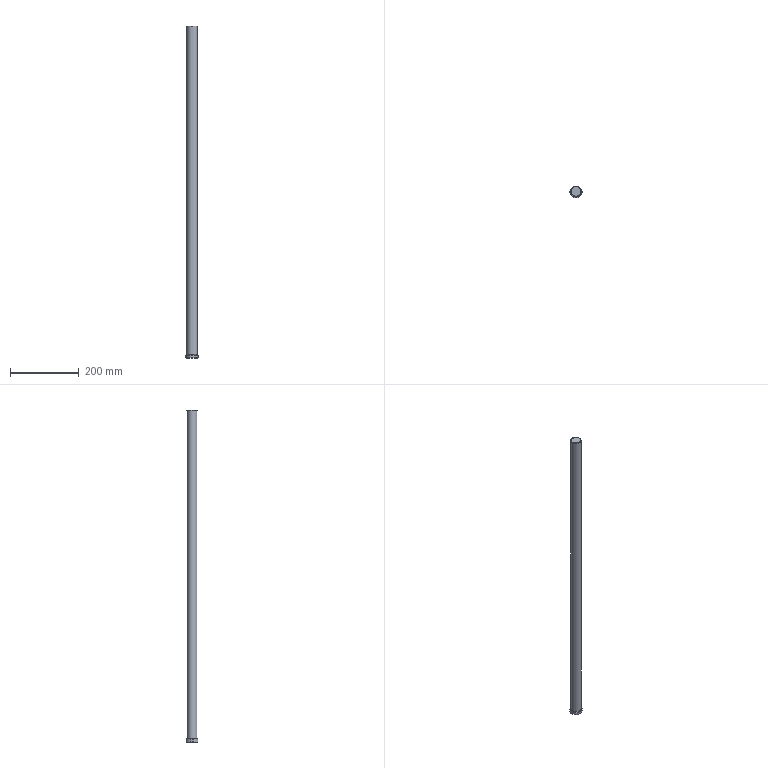Part | STEP file | solid 29 | 1 solid | 15 faces | box 35 x 35 x 965 mm | volume 683981 mm3 | plane 6 | cylinder 3 | torus 2 | cone 2 | other 1 | spline 1 | commonest cylinder face diameters 30 x2 35 x1